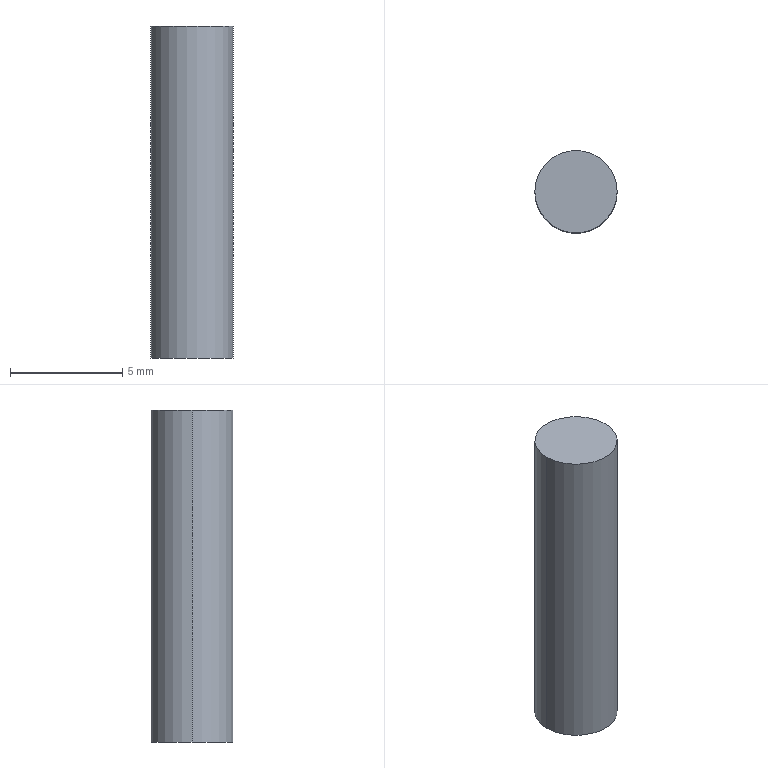Part | SolidWorks | features BaseBody 1 | 1 solid | 4 faces | box 3.663 x 3.663 x 14.762 mm | volume 155.592 mm3 | cylinder 2 | plane 2 | commonest cylinder face diameters 3.663 x2
STEP:
#1=CARTESIAN_POINT('',(-181.411,-39.199,-7.381));
#2=VERTEX_POINT('',#1);
#3=CARTESIAN_POINT('',(-185.074,-39.199,-7.381));
#4=VERTEX_POINT('',#3);
#5=CARTESIAN_POINT('',(-183.243,-39.199,-7.381));
#6=DIRECTION('',(0.,0.,1.));
#7=DIRECTION('',(1.,0.,0.));
#8=AXIS2_PLACEMENT_3D('',#5,#6,#7);
#9=CIRCLE('',#8,1.832);
#10=EDGE_CURVE('',#2,#4,#9,.T.);
#11=ORIENTED_EDGE('',*,*,#10,.T.);
#12=CARTESIAN_POINT('',(-185.074,-39.199,7.381));
#13=VERTEX_POINT('',#12);
#14=CARTESIAN_POINT('',(-185.074,-39.199,0.));
#15=DIRECTION('',(0.,0.,1.));
#16=VECTOR('',#15,1000.);
#17=LINE('',#14,#16);
#18=EDGE_CURVE('',#4,#13,#17,.T.);
#19=ORIENTED_EDGE('',*,*,#18,.T.);
#20=CARTESIAN_POINT('',(-181.411,-39.199,7.381));
#21=VERTEX_POINT('',#20);
#22=CARTESIAN_POINT('',(-183.243,-39.199,7.381));
#23=DIRECTION('',(0.,0.,-1.));
#24=DIRECTION('',(1.,0.,0.));
#25=AXIS2_PLACEMENT_3D('',#22,#23,#24);
#26=CIRCLE('',#25,1.832);
#27=EDGE_CURVE('',#13,#21,#26,.T.);
#28=ORIENTED_EDGE('',*,*,#27,.T.);
#29=CARTESIAN_POINT('',(-181.411,-39.199,0.));
#30=DIRECTION('',(0.,0.,1.));
#31=VECTOR('',#30,1000.);
#32=LINE('',#29,#31);
#33=EDGE_CURVE('',#2,#21,#32,.T.);
#34=ORIENTED_EDGE('',*,*,#33,.F.);
#35=EDGE_LOOP('',(#11,#19,#28,#34));
#36=FACE_OUTER_BOUND('',#35,.T.);
#37=CARTESIAN_POINT('',(-183.243,-39.199,0.));
#38=DIRECTION('',(0.,0.,1.));
#39=DIRECTION('',(1.,0.,0.));
#40=AXIS2_PLACEMENT_3D('',#37,#38,#39);
#41=CYLINDRICAL_SURFACE('',#40,1.832);
#42=ADVANCED_FACE('',(#36),#41,.T.);
#43=ORIENTED_EDGE('',*,*,#18,.F.);
#44=CARTESIAN_POINT('',(-183.243,-39.199,-7.381));
#45=DIRECTION('',(0.,0.,1.));
#46=DIRECTION('',(1.,0.,0.));
#47=AXIS2_PLACEMENT_3D('',#44,#45,#46);
#48=CIRCLE('',#47,1.832);
#49=EDGE_CURVE('',#4,#2,#48,.T.);
#50=ORIENTED_EDGE('',*,*,#49,.T.);
#51=ORIENTED_EDGE('',*,*,#33,.T.);
#52=CARTESIAN_POINT('',(-183.243,-39.199,7.381));
#53=DIRECTION('',(0.,0.,-1.));
#54=DIRECTION('',(1.,0.,0.));
#55=AXIS2_PLACEMENT_3D('',#52,#53,#54);
#56=CIRCLE('',#55,1.832);
#57=EDGE_CURVE('',#21,#13,#56,.T.);
#58=ORIENTED_EDGE('',*,*,#57,.T.);
#59=EDGE_LOOP('',(#43,#50,#51,#58));
#60=FACE_OUTER_BOUND('',#59,.T.);
#61=CARTESIAN_POINT('',(-183.243,-39.199,0.));
#62=DIRECTION('',(0.,0.,1.));
#63=DIRECTION('',(1.,0.,0.));
#64=AXIS2_PLACEMENT_3D('',#61,#62,#63);
#65=CYLINDRICAL_SURFACE('',#64,1.832);
#66=ADVANCED_FACE('',(#60),#65,.T.);
#67=ORIENTED_EDGE('',*,*,#10,.F.);
#68=ORIENTED_EDGE('',*,*,#49,.F.);
#69=EDGE_LOOP('',(#67,#68));
#70=FACE_OUTER_BOUND('',#69,.T.);
#71=CARTESIAN_POINT('',(-183.243,-39.199,-7.381));
#72=DIRECTION('',(0.,0.,1.));
#73=DIRECTION('',(1.,0.,0.));
#74=AXIS2_PLACEMENT_3D('',#71,#72,#73);
#75=PLANE('',#74);
#76=ADVANCED_FACE('',(#70),#75,.F.);
#77=ORIENTED_EDGE('',*,*,#57,.F.);
#78=ORIENTED_EDGE('',*,*,#27,.F.);
#79=EDGE_LOOP('',(#77,#78));
#80=FACE_OUTER_BOUND('',#79,.T.);
#81=CARTESIAN_POINT('',(-183.243,-39.199,7.381));
#82=DIRECTION('',(0.,0.,1.));
#83=DIRECTION('',(1.,0.,0.));
#84=AXIS2_PLACEMENT_3D('',#81,#82,#83);
#85=PLANE('',#84);
#86=ADVANCED_FACE('',(#80),#85,.T.);
#87=CLOSED_SHELL('',(#42,#66,#76,#86));
#88=MANIFOLD_SOLID_BREP('',#87);
#89=CARTESIAN_POINT('',(0.,0.,0.));
#90=DIRECTION('',(0.,0.,1.));
#91=DIRECTION('',(1.,0.,0.));
#92=AXIS2_PLACEMENT_3D('',#89,#90,#91);
#93=(LENGTH_UNIT()NAMED_UNIT(*)SI_UNIT(.MILLI.,.METRE.));
#94=UNCERTAINTY_MEASURE_WITH_UNIT(LENGTH_MEASURE(0.00001),#93,'','');
#95=(NAMED_UNIT(*)PLANE_ANGLE_UNIT()SI_UNIT($,.RADIAN.));
#96=(NAMED_UNIT(*)SI_UNIT($,.STERADIAN.)SOLID_ANGLE_UNIT());
#97=(GEOMETRIC_REPRESENTATION_CONTEXT(3)GLOBAL_UNCERTAINTY_ASSIGNED_CONTEXT((#94))GLOBAL_UNIT_ASSIGNED_CONTEXT((#93,#95,#96))REPRESENTATION_CONTEXT('',''));
#98=ADVANCED_BREP_SHAPE_REPRESENTATION('',(#88,#92),#97);